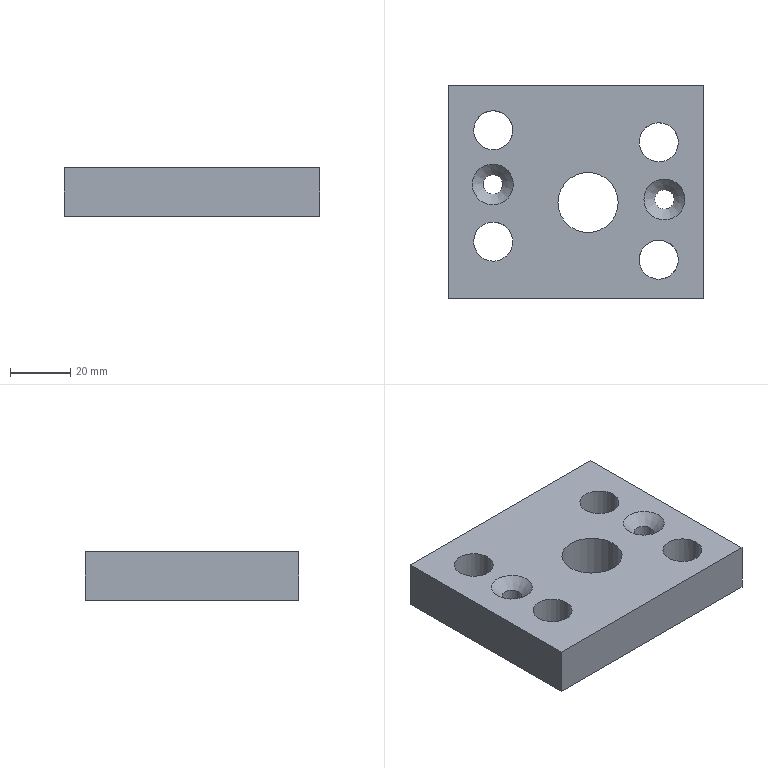Part | STEP file | gslz 2016.10.28-13_id1610_x_t | 1 solid | 15 faces | box 85 x 71 x 16 mm | volume 81626 mm3 | cylinder 7 | plane 6 | cone 2 | commonest cylinder face diameters 13 x4 6.5 x2 20 x1
STEP:
#1=CARTESIAN_POINT('',(0.,0.,0.));
#2=DIRECTION('',(0.,0.,1.));
#3=DIRECTION('',(1.,0.,0.));
#4=AXIS2_PLACEMENT_3D('',#1,#2,#3);
#5=CARTESIAN_POINT('',(-1398.441,280.34,-48.));
#6=VERTEX_POINT('',#5);
#7=CARTESIAN_POINT('',(-1399.872,274.,-48.));
#8=DIRECTION('',(0.,0.,1.));
#9=DIRECTION('',(0.2202,0.9754,0.));
#10=AXIS2_PLACEMENT_3D('',#7,#8,#9);
#11=CIRCLE('',#10,6.5);
#12=CARTESIAN_POINT('',(-1345.502,255.485,-48.));
#13=DIRECTION('',(0.,0.,1.));
#14=DIRECTION('',(1.,0.,0.));
#15=AXIS2_PLACEMENT_3D('',#12,#13,#14);
#16=PLANE('',#15);
#17=CARTESIAN_POINT('',(-54.371,18.515));
#18=DIRECTION('',(0.2202,0.9754));
#19=AXIS2_PLACEMENT_2D('',#17,#18);
#20=CIRCLE('',#19,6.5);
#21=(GEOMETRIC_REPRESENTATION_CONTEXT(2)PARAMETRIC_REPRESENTATION_CONTEXT()REPRESENTATION_CONTEXT('',''));
#22=DEFINITIONAL_REPRESENTATION('',(#20),#21);
#23=PCURVE('',#16,#22);
#24=CARTESIAN_POINT('',(-1399.872,274.,-95.));
#25=DIRECTION('',(0.,0.,1.));
#26=DIRECTION('',(-0.2202,-0.9754,0.));
#27=AXIS2_PLACEMENT_3D('',#24,#25,#26);
#28=CYLINDRICAL_SURFACE('',#27,6.5);
#29=CARTESIAN_POINT('',(3.142,47.));
#30=DIRECTION('',(1.,0.));
#31=VECTOR('',#30,1.);
#32=LINE('',#29,#31);
#33=(GEOMETRIC_REPRESENTATION_CONTEXT(2)PARAMETRIC_REPRESENTATION_CONTEXT()REPRESENTATION_CONTEXT('',''));
#34=DEFINITIONAL_REPRESENTATION('',(#32),#33);
#35=PCURVE('',#28,#34);
#36=SURFACE_CURVE('',#11,(#23,#35),.PCURVE_S1.);
#37=EDGE_CURVE('',#6,#6,#36,.T.);
#38=ORIENTED_EDGE('',*,*,#37,.T.);
#39=EDGE_LOOP('',(#38));
#40=FACE_BOUND('',#39,.T.);
#41=CARTESIAN_POINT('',(-1455.963,271.592,-48.));
#42=VERTEX_POINT('',#41);
#43=CARTESIAN_POINT('',(-1454.872,278.,-48.));
#44=DIRECTION('',(0.,0.,1.));
#45=DIRECTION('',(-0.1678,-0.9858,0.));
#46=AXIS2_PLACEMENT_3D('',#43,#44,#45);
#47=CIRCLE('',#46,6.5);
#48=CARTESIAN_POINT('',(-109.371,22.515));
#49=DIRECTION('',(-0.1678,-0.9858));
#50=AXIS2_PLACEMENT_2D('',#48,#49);
#51=CIRCLE('',#50,6.5);
#52=(GEOMETRIC_REPRESENTATION_CONTEXT(2)PARAMETRIC_REPRESENTATION_CONTEXT()REPRESENTATION_CONTEXT('',''));
#53=DEFINITIONAL_REPRESENTATION('',(#51),#52);
#54=PCURVE('',#16,#53);
#55=CARTESIAN_POINT('',(-1454.872,278.,-0.5408));
#56=DIRECTION('',(0.,0.,-1.));
#57=DIRECTION('',(-1.,0.,0.));
#58=AXIS2_PLACEMENT_3D('',#55,#56,#57);
#59=CYLINDRICAL_SURFACE('',#58,6.5);
#60=CARTESIAN_POINT('',(11.164,47.459));
#61=DIRECTION('',(-1.,0.));
#62=VECTOR('',#61,1.);
#63=LINE('',#60,#62);
#64=(GEOMETRIC_REPRESENTATION_CONTEXT(2)PARAMETRIC_REPRESENTATION_CONTEXT()REPRESENTATION_CONTEXT('',''));
#65=DEFINITIONAL_REPRESENTATION('',(#63),#64);
#66=PCURVE('',#59,#65);
#67=SURFACE_CURVE('',#47,(#54,#66),.PCURVE_S1.);
#68=EDGE_CURVE('',#42,#42,#67,.T.);
#69=ORIENTED_EDGE('',*,*,#68,.T.);
#70=EDGE_LOOP('',(#69));
#71=FACE_BOUND('',#70,.T.);
#72=CARTESIAN_POINT('',(-1394.75,255.,-48.));
#73=VERTEX_POINT('',#72);
#74=CARTESIAN_POINT('',(-1398.,255.,-48.));
#75=DIRECTION('',(0.,0.,-1.));
#76=DIRECTION('',(1.,0.,0.));
#77=AXIS2_PLACEMENT_3D('',#74,#75,#76);
#78=CIRCLE('',#77,3.25);
#79=CARTESIAN_POINT('',(-49.248,-0.4849));
#80=CARTESIAN_POINT('',(-49.248,-6.114));
#81=CARTESIAN_POINT('',(-54.123,-3.299));
#82=CARTESIAN_POINT('',(-58.998,-0.4849));
#83=CARTESIAN_POINT('',(-54.123,2.33));
#84=CARTESIAN_POINT('',(-49.248,5.144));
#85=CARTESIAN_POINT('',(-49.248,-0.4849));
#86=(BOUNDED_CURVE()B_SPLINE_CURVE(2,(#79,#80,#81,#82,#83,#84,#85),.UNSPECIFIED.,.T.,.F.)B_SPLINE_CURVE_WITH_KNOTS((1,2,2,2,2,1),(-2.094,0.,2.094,4.189,6.283,8.378),.UNSPECIFIED.)CURVE()GEOMETRIC_REPRESENTATION_ITEM()RATIONAL_B_SPLINE_CURVE((1.,0.5,1.,0.5,1.,0.5,1.))REPRESENTATION_ITEM(''));
#87=(GEOMETRIC_REPRESENTATION_CONTEXT(2)PARAMETRIC_REPRESENTATION_CONTEXT()REPRESENTATION_CONTEXT('',''));
#88=DEFINITIONAL_REPRESENTATION('',(#86),#87);
#89=PCURVE('',#16,#88);
#90=CARTESIAN_POINT('',(-1398.,255.,-32.));
#91=DIRECTION('',(0.,0.,-1.));
#92=DIRECTION('',(-1.,0.,0.));
#93=AXIS2_PLACEMENT_3D('',#90,#91,#92);
#94=CYLINDRICAL_SURFACE('',#93,3.25);
#95=CARTESIAN_POINT('',(3.142,16.));
#96=DIRECTION('',(1.,0.));
#97=VECTOR('',#96,1.);
#98=LINE('',#95,#97);
#99=(GEOMETRIC_REPRESENTATION_CONTEXT(2)PARAMETRIC_REPRESENTATION_CONTEXT()REPRESENTATION_CONTEXT('',''));
#100=DEFINITIONAL_REPRESENTATION('',(#98),#99);
#101=PCURVE('',#94,#100);
#102=SURFACE_CURVE('',#78,(#89,#101),.PCURVE_S1.);
#103=EDGE_CURVE('',#73,#73,#102,.T.);
#104=ORIENTED_EDGE('',*,*,#103,.F.);
#105=EDGE_LOOP('',(#104));
#106=FACE_BOUND('',#105,.T.);
#107=CARTESIAN_POINT('',(-1451.75,260.,-48.));
#108=VERTEX_POINT('',#107);
#109=CARTESIAN_POINT('',(-1455.,260.,-48.));
#110=DIRECTION('',(0.,0.,-1.));
#111=DIRECTION('',(1.,0.,0.));
#112=AXIS2_PLACEMENT_3D('',#109,#110,#111);
#113=CIRCLE('',#112,3.25);
#114=CARTESIAN_POINT('',(-106.248,4.515));
#115=CARTESIAN_POINT('',(-106.248,-1.114));
#116=CARTESIAN_POINT('',(-111.123,1.701));
#117=CARTESIAN_POINT('',(-115.998,4.515));
#118=CARTESIAN_POINT('',(-111.123,7.33));
#119=CARTESIAN_POINT('',(-106.248,10.144));
#120=CARTESIAN_POINT('',(-106.248,4.515));
#121=(BOUNDED_CURVE()B_SPLINE_CURVE(2,(#114,#115,#116,#117,#118,#119,#120),.UNSPECIFIED.,.T.,.F.)B_SPLINE_CURVE_WITH_KNOTS((1,2,2,2,2,1),(-2.094,0.,2.094,4.189,6.283,8.378),.UNSPECIFIED.)CURVE()GEOMETRIC_REPRESENTATION_ITEM()RATIONAL_B_SPLINE_CURVE((1.,0.5,1.,0.5,1.,0.5,1.))REPRESENTATION_ITEM(''));
#122=(GEOMETRIC_REPRESENTATION_CONTEXT(2)PARAMETRIC_REPRESENTATION_CONTEXT()REPRESENTATION_CONTEXT('',''));
#123=DEFINITIONAL_REPRESENTATION('',(#121),#122);
#124=PCURVE('',#16,#123);
#125=CARTESIAN_POINT('',(-1455.,260.,-32.));
#126=DIRECTION('',(0.,0.,-1.));
#127=DIRECTION('',(-1.,0.,0.));
#128=AXIS2_PLACEMENT_3D('',#125,#126,#127);
#129=CYLINDRICAL_SURFACE('',#128,3.25);
#130=CARTESIAN_POINT('',(3.142,16.));
#131=DIRECTION('',(1.,0.));
#132=VECTOR('',#131,1.);
#133=LINE('',#130,#132);
#134=(GEOMETRIC_REPRESENTATION_CONTEXT(2)PARAMETRIC_REPRESENTATION_CONTEXT()REPRESENTATION_CONTEXT('',''));
#135=DEFINITIONAL_REPRESENTATION('',(#133),#134);
#136=PCURVE('',#129,#135);
#137=SURFACE_CURVE('',#113,(#124,#136),.PCURVE_S1.);
#138=EDGE_CURVE('',#108,#108,#137,.T.);
#139=ORIENTED_EDGE('',*,*,#138,.F.);
#140=EDGE_LOOP('',(#139));
#141=FACE_BOUND('',#140,.T.);
#142=CARTESIAN_POINT('',(-1469.872,293.,-48.));
#143=VERTEX_POINT('',#142);
#144=CARTESIAN_POINT('',(-1469.872,222.,-48.));
#145=VERTEX_POINT('',#144);
#146=CARTESIAN_POINT('',(-1469.872,336.,-48.));
#147=DIRECTION('',(0.,-1.,0.));
#148=VECTOR('',#147,1.);
#149=LINE('',#146,#148);
#150=CARTESIAN_POINT('',(-124.371,80.515));
#151=DIRECTION('',(0.,-1.));
#152=VECTOR('',#151,1.);
#153=LINE('',#150,#152);
#154=(GEOMETRIC_REPRESENTATION_CONTEXT(2)PARAMETRIC_REPRESENTATION_CONTEXT()REPRESENTATION_CONTEXT('',''));
#155=DEFINITIONAL_REPRESENTATION('',(#153),#154);
#156=PCURVE('',#16,#155);
#157=CARTESIAN_POINT('',(-1469.872,336.,-40.));
#158=DIRECTION('',(-1.,0.,0.));
#159=DIRECTION('',(0.,0.,1.));
#160=AXIS2_PLACEMENT_3D('',#157,#158,#159);
#161=PLANE('',#160);
#162=CARTESIAN_POINT('',(-8.,0.));
#163=DIRECTION('',(0.,-1.));
#164=VECTOR('',#163,1.);
#165=LINE('',#162,#164);
#166=(GEOMETRIC_REPRESENTATION_CONTEXT(2)PARAMETRIC_REPRESENTATION_CONTEXT()REPRESENTATION_CONTEXT('',''));
#167=DEFINITIONAL_REPRESENTATION('',(#165),#166);
#168=PCURVE('',#161,#167);
#169=SURFACE_CURVE('',#149,(#156,#168),.PCURVE_S1.);
#170=EDGE_CURVE('',#143,#145,#169,.T.);
#171=ORIENTED_EDGE('',*,*,#170,.F.);
#172=CARTESIAN_POINT('',(-1384.872,293.,-48.));
#173=VERTEX_POINT('',#172);
#174=CARTESIAN_POINT('',(-1423.372,293.,-48.));
#175=DIRECTION('',(-1.,0.,0.));
#176=VECTOR('',#175,1.);
#177=LINE('',#174,#176);
#178=CARTESIAN_POINT('',(-77.871,37.515));
#179=DIRECTION('',(-1.,0.));
#180=VECTOR('',#179,1.);
#181=LINE('',#178,#180);
#182=(GEOMETRIC_REPRESENTATION_CONTEXT(2)PARAMETRIC_REPRESENTATION_CONTEXT()REPRESENTATION_CONTEXT('',''));
#183=DEFINITIONAL_REPRESENTATION('',(#181),#182);
#184=PCURVE('',#16,#183);
#185=CARTESIAN_POINT('',(-1423.372,293.,-40.));
#186=DIRECTION('',(0.,1.,0.));
#187=DIRECTION('',(0.,0.,1.));
#188=AXIS2_PLACEMENT_3D('',#185,#186,#187);
#189=PLANE('',#188);
#190=CARTESIAN_POINT('',(-8.,0.));
#191=DIRECTION('',(0.,-1.));
#192=VECTOR('',#191,1.);
#193=LINE('',#190,#192);
#194=(GEOMETRIC_REPRESENTATION_CONTEXT(2)PARAMETRIC_REPRESENTATION_CONTEXT()REPRESENTATION_CONTEXT('',''));
#195=DEFINITIONAL_REPRESENTATION('',(#193),#194);
#196=PCURVE('',#189,#195);
#197=SURFACE_CURVE('',#177,(#184,#196),.PCURVE_S1.);
#198=EDGE_CURVE('',#173,#143,#197,.T.);
#199=ORIENTED_EDGE('',*,*,#198,.F.);
#200=CARTESIAN_POINT('',(-1384.872,222.,-48.));
#201=VERTEX_POINT('',#200);
#202=CARTESIAN_POINT('',(-1384.872,336.,-48.));
#203=DIRECTION('',(0.,1.,0.));
#204=VECTOR('',#203,1.);
#205=LINE('',#202,#204);
#206=CARTESIAN_POINT('',(-39.371,80.515));
#207=DIRECTION('',(0.,1.));
#208=VECTOR('',#207,1.);
#209=LINE('',#206,#208);
#210=(GEOMETRIC_REPRESENTATION_CONTEXT(2)PARAMETRIC_REPRESENTATION_CONTEXT()REPRESENTATION_CONTEXT('',''));
#211=DEFINITIONAL_REPRESENTATION('',(#209),#210);
#212=PCURVE('',#16,#211);
#213=CARTESIAN_POINT('',(-1384.872,336.,-40.));
#214=DIRECTION('',(1.,0.,0.));
#215=DIRECTION('',(0.,0.,-1.));
#216=AXIS2_PLACEMENT_3D('',#213,#214,#215);
#217=PLANE('',#216);
#218=CARTESIAN_POINT('',(8.,0.));
#219=DIRECTION('',(0.,1.));
#220=VECTOR('',#219,1.);
#221=LINE('',#218,#220);
#222=(GEOMETRIC_REPRESENTATION_CONTEXT(2)PARAMETRIC_REPRESENTATION_CONTEXT()REPRESENTATION_CONTEXT('',''));
#223=DEFINITIONAL_REPRESENTATION('',(#221),#222);
#224=PCURVE('',#217,#223);
#225=SURFACE_CURVE('',#205,(#212,#224),.PCURVE_S1.);
#226=EDGE_CURVE('',#201,#173,#225,.T.);
#227=ORIENTED_EDGE('',*,*,#226,.F.);
#228=CARTESIAN_POINT('',(-1423.372,222.,-48.));
#229=DIRECTION('',(1.,0.,0.));
#230=VECTOR('',#229,1.);
#231=LINE('',#228,#230);
#232=CARTESIAN_POINT('',(-77.871,-33.485));
#233=DIRECTION('',(1.,0.));
#234=VECTOR('',#233,1.);
#235=LINE('',#232,#234);
#236=(GEOMETRIC_REPRESENTATION_CONTEXT(2)PARAMETRIC_REPRESENTATION_CONTEXT()REPRESENTATION_CONTEXT('',''));
#237=DEFINITIONAL_REPRESENTATION('',(#235),#236);
#238=PCURVE('',#16,#237);
#239=CARTESIAN_POINT('',(-1423.372,222.,-40.));
#240=DIRECTION('',(0.,-1.,0.));
#241=DIRECTION('',(0.,0.,-1.));
#242=AXIS2_PLACEMENT_3D('',#239,#240,#241);
#243=PLANE('',#242);
#244=CARTESIAN_POINT('',(8.,0.));
#245=DIRECTION('',(0.,1.));
#246=VECTOR('',#245,1.);
#247=LINE('',#244,#246);
#248=(GEOMETRIC_REPRESENTATION_CONTEXT(2)PARAMETRIC_REPRESENTATION_CONTEXT()REPRESENTATION_CONTEXT('',''));
#249=DEFINITIONAL_REPRESENTATION('',(#247),#248);
#250=PCURVE('',#243,#249);
#251=SURFACE_CURVE('',#231,(#238,#250),.PCURVE_S1.);
#252=EDGE_CURVE('',#145,#201,#251,.T.);
#253=ORIENTED_EDGE('',*,*,#252,.F.);
#254=EDGE_LOOP('',(#171,#199,#227,#253));
#255=FACE_BOUND('',#254,.T.);
#256=CARTESIAN_POINT('',(-1413.372,254.,-48.));
#257=VERTEX_POINT('',#256);
#258=CARTESIAN_POINT('',(-1423.372,254.,-48.));
#259=DIRECTION('',(0.,0.,-1.));
#260=DIRECTION('',(1.,0.,0.));
#261=AXIS2_PLACEMENT_3D('',#258,#259,#260);
#262=CIRCLE('',#261,10.);
#263=CARTESIAN_POINT('',(-67.871,-1.485));
#264=CARTESIAN_POINT('',(-67.871,-18.805));
#265=CARTESIAN_POINT('',(-82.871,-10.145));
#266=CARTESIAN_POINT('',(-97.871,-1.485));
#267=CARTESIAN_POINT('',(-82.871,7.175));
#268=CARTESIAN_POINT('',(-67.871,15.836));
#269=CARTESIAN_POINT('',(-67.871,-1.485));
#270=(BOUNDED_CURVE()B_SPLINE_CURVE(2,(#263,#264,#265,#266,#267,#268,#269),.UNSPECIFIED.,.T.,.F.)B_SPLINE_CURVE_WITH_KNOTS((1,2,2,2,2,1),(-2.094,0.,2.094,4.189,6.283,8.378),.UNSPECIFIED.)CURVE()GEOMETRIC_REPRESENTATION_ITEM()RATIONAL_B_SPLINE_CURVE((1.,0.5,1.,0.5,1.,0.5,1.))REPRESENTATION_ITEM(''));
#271=(GEOMETRIC_REPRESENTATION_CONTEXT(2)PARAMETRIC_REPRESENTATION_CONTEXT()REPRESENTATION_CONTEXT('',''));
#272=DEFINITIONAL_REPRESENTATION('',(#270),#271);
#273=PCURVE('',#16,#272);
#274=CARTESIAN_POINT('',(-1423.372,254.,-257.));
#275=DIRECTION('',(0.,0.,1.));
#276=DIRECTION('',(1.,0.,0.));
#277=AXIS2_PLACEMENT_3D('',#274,#275,#276);
#278=CYLINDRICAL_SURFACE('',#277,10.);
#279=CARTESIAN_POINT('',(6.283,209.));
#280=DIRECTION('',(-1.,0.));
#281=VECTOR('',#280,1.);
#282=LINE('',#279,#281);
#283=(GEOMETRIC_REPRESENTATION_CONTEXT(2)PARAMETRIC_REPRESENTATION_CONTEXT()REPRESENTATION_CONTEXT('',''));
#284=DEFINITIONAL_REPRESENTATION('',(#282),#283);
#285=PCURVE('',#278,#284);
#286=SURFACE_CURVE('',#262,(#273,#285),.PCURVE_S1.);
#287=EDGE_CURVE('',#257,#257,#286,.T.);
#288=ORIENTED_EDGE('',*,*,#287,.F.);
#289=EDGE_LOOP('',(#288));
#290=FACE_BOUND('',#289,.T.);
#291=CARTESIAN_POINT('',(-1453.441,247.34,-48.));
#292=VERTEX_POINT('',#291);
#293=CARTESIAN_POINT('',(-1454.872,241.,-48.));
#294=DIRECTION('',(0.,0.,1.));
#295=DIRECTION('',(0.2202,0.9754,0.));
#296=AXIS2_PLACEMENT_3D('',#293,#294,#295);
#297=CIRCLE('',#296,6.5);
#298=CARTESIAN_POINT('',(-109.371,-14.485));
#299=DIRECTION('',(0.2202,0.9754));
#300=AXIS2_PLACEMENT_2D('',#298,#299);
#301=CIRCLE('',#300,6.5);
#302=(GEOMETRIC_REPRESENTATION_CONTEXT(2)PARAMETRIC_REPRESENTATION_CONTEXT()REPRESENTATION_CONTEXT('',''));
#303=DEFINITIONAL_REPRESENTATION('',(#301),#302);
#304=PCURVE('',#16,#303);
#305=CARTESIAN_POINT('',(-1454.872,241.,-95.));
#306=DIRECTION('',(0.,0.,1.));
#307=DIRECTION('',(-0.2202,-0.9754,0.));
#308=AXIS2_PLACEMENT_3D('',#305,#306,#307);
#309=CYLINDRICAL_SURFACE('',#308,6.5);
#310=CARTESIAN_POINT('',(3.142,47.));
#311=DIRECTION('',(1.,0.));
#312=VECTOR('',#311,1.);
#313=LINE('',#310,#312);
#314=(GEOMETRIC_REPRESENTATION_CONTEXT(2)PARAMETRIC_REPRESENTATION_CONTEXT()REPRESENTATION_CONTEXT('',''));
#315=DEFINITIONAL_REPRESENTATION('',(#313),#314);
#316=PCURVE('',#309,#315);
#317=SURFACE_CURVE('',#297,(#304,#316),.PCURVE_S1.);
#318=EDGE_CURVE('',#292,#292,#317,.T.);
#319=ORIENTED_EDGE('',*,*,#318,.T.);
#320=EDGE_LOOP('',(#319));
#321=FACE_BOUND('',#320,.T.);
#322=CARTESIAN_POINT('',(-1400.963,228.592,-48.));
#323=VERTEX_POINT('',#322);
#324=CARTESIAN_POINT('',(-1399.872,235.,-48.));
#325=DIRECTION('',(0.,0.,1.));
#326=DIRECTION('',(-0.1678,-0.9858,0.));
#327=AXIS2_PLACEMENT_3D('',#324,#325,#326);
#328=CIRCLE('',#327,6.5);
#329=CARTESIAN_POINT('',(-54.371,-20.485));
#330=DIRECTION('',(-0.1678,-0.9858));
#331=AXIS2_PLACEMENT_2D('',#329,#330);
#332=CIRCLE('',#331,6.5);
#333=(GEOMETRIC_REPRESENTATION_CONTEXT(2)PARAMETRIC_REPRESENTATION_CONTEXT()REPRESENTATION_CONTEXT('',''));
#334=DEFINITIONAL_REPRESENTATION('',(#332),#333);
#335=PCURVE('',#16,#334);
#336=CARTESIAN_POINT('',(-1399.872,235.,-0.5408));
#337=DIRECTION('',(0.,0.,-1.));
#338=DIRECTION('',(-1.,0.,0.));
#339=AXIS2_PLACEMENT_3D('',#336,#337,#338);
#340=CYLINDRICAL_SURFACE('',#339,6.5);
#341=CARTESIAN_POINT('',(11.164,47.459));
#342=DIRECTION('',(-1.,0.));
#343=VECTOR('',#342,1.);
#344=LINE('',#341,#343);
#345=(GEOMETRIC_REPRESENTATION_CONTEXT(2)PARAMETRIC_REPRESENTATION_CONTEXT()REPRESENTATION_CONTEXT('',''));
#346=DEFINITIONAL_REPRESENTATION('',(#344),#345);
#347=PCURVE('',#340,#346);
#348=SURFACE_CURVE('',#328,(#335,#347),.PCURVE_S1.);
#349=EDGE_CURVE('',#323,#323,#348,.T.);
#350=ORIENTED_EDGE('',*,*,#349,.T.);
#351=EDGE_LOOP('',(#350));
#352=FACE_BOUND('',#351,.T.);
#353=ADVANCED_FACE('',(#40,#71,#106,#141,#255,#290,#321,#352),#16,.F.);
#354=CARTESIAN_POINT('',(-1393.372,235.,-32.));
#355=VERTEX_POINT('',#354);
#356=CARTESIAN_POINT('',(-1400.963,228.592,-32.));
#357=VERTEX_POINT('',#356);
#358=CARTESIAN_POINT('',(-1399.872,235.,-32.));
#359=DIRECTION('',(0.,0.,-1.));
#360=DIRECTION('',(1.,0.,0.));
#361=AXIS2_PLACEMENT_3D('',#358,#359,#360);
#362=CIRCLE('',#361,6.5);
#363=CARTESIAN_POINT('',(-1345.502,255.485,-32.));
#364=DIRECTION('',(0.,0.,1.));
#365=DIRECTION('',(1.,0.,0.));
#366=AXIS2_PLACEMENT_3D('',#363,#364,#365);
#367=PLANE('',#366);
#368=CARTESIAN_POINT('',(-47.871,-20.485));
#369=CARTESIAN_POINT('',(-47.871,-31.743));
#370=CARTESIAN_POINT('',(-57.621,-26.114));
#371=CARTESIAN_POINT('',(-67.371,-20.485));
#372=CARTESIAN_POINT('',(-57.621,-14.856));
#373=CARTESIAN_POINT('',(-47.871,-9.227));
#374=CARTESIAN_POINT('',(-47.871,-20.485));
#375=(BOUNDED_CURVE()B_SPLINE_CURVE(2,(#368,#369,#370,#371,#372,#373,#374),.UNSPECIFIED.,.T.,.F.)B_SPLINE_CURVE_WITH_KNOTS((1,2,2,2,2,1),(-2.094,0.,2.094,4.189,6.283,8.378),.UNSPECIFIED.)CURVE()GEOMETRIC_REPRESENTATION_ITEM()RATIONAL_B_SPLINE_CURVE((1.,0.5,1.,0.5,1.,0.5,1.))REPRESENTATION_ITEM(''));
#376=(GEOMETRIC_REPRESENTATION_CONTEXT(2)PARAMETRIC_REPRESENTATION_CONTEXT()REPRESENTATION_CONTEXT('',''));
#377=DEFINITIONAL_REPRESENTATION('',(#375),#376);
#378=PCURVE('',#367,#377);
#379=CARTESIAN_POINT('',(9.425,31.459));
#380=DIRECTION('',(1.,0.));
#381=VECTOR('',#380,1.);
#382=LINE('',#379,#381);
#383=(GEOMETRIC_REPRESENTATION_CONTEXT(2)PARAMETRIC_REPRESENTATION_CONTEXT()REPRESENTATION_CONTEXT('',''));
#384=DEFINITIONAL_REPRESENTATION('',(#382),#383);
#385=PCURVE('',#340,#384);
#386=SURFACE_CURVE('',#362,(#378,#385),.PCURVE_S1.);
#387=EDGE_CURVE('',#355,#357,#386,.T.);
#388=ORIENTED_EDGE('',*,*,#387,.T.);
#389=CARTESIAN_POINT('',(-1399.872,235.,-32.));
#390=DIRECTION('',(0.,0.,-1.));
#391=DIRECTION('',(1.,0.,0.));
#392=AXIS2_PLACEMENT_3D('',#389,#390,#391);
#393=CIRCLE('',#392,6.5);
#394=CARTESIAN_POINT('',(-47.871,-20.485));
#395=CARTESIAN_POINT('',(-47.871,-31.743));
#396=CARTESIAN_POINT('',(-57.621,-26.114));
#397=CARTESIAN_POINT('',(-67.371,-20.485));
#398=CARTESIAN_POINT('',(-57.621,-14.856));
#399=CARTESIAN_POINT('',(-47.871,-9.227));
#400=CARTESIAN_POINT('',(-47.871,-20.485));
#401=(BOUNDED_CURVE()B_SPLINE_CURVE(2,(#394,#395,#396,#397,#398,#399,#400),.UNSPECIFIED.,.T.,.F.)B_SPLINE_CURVE_WITH_KNOTS((1,2,2,2,2,1),(-2.094,0.,2.094,4.189,6.283,8.378),.UNSPECIFIED.)CURVE()GEOMETRIC_REPRESENTATION_ITEM()RATIONAL_B_SPLINE_CURVE((1.,0.5,1.,0.5,1.,0.5,1.))REPRESENTATION_ITEM(''));
#402=(GEOMETRIC_REPRESENTATION_CONTEXT(2)PARAMETRIC_REPRESENTATION_CONTEXT()REPRESENTATION_CONTEXT('',''));
#403=DEFINITIONAL_REPRESENTATION('',(#401),#402);
#404=PCURVE('',#367,#403);
#405=CARTESIAN_POINT('',(3.142,31.459));
#406=DIRECTION('',(1.,0.));
#407=VECTOR('',#406,1.);
#408=LINE('',#405,#407);
#409=(GEOMETRIC_REPRESENTATION_CONTEXT(2)PARAMETRIC_REPRESENTATION_CONTEXT()REPRESENTATION_CONTEXT('',''));
#410=DEFINITIONAL_REPRESENTATION('',(#408),#409);
#411=PCURVE('',#340,#410);
#412=SURFACE_CURVE('',#393,(#404,#411),.PCURVE_S1.);
#413=EDGE_CURVE('',#357,#355,#412,.T.);
#414=ORIENTED_EDGE('',*,*,#413,.T.);
#415=EDGE_LOOP('',(#388,#414));
#416=FACE_BOUND('',#415,.T.);
#417=CARTESIAN_POINT('',(-1398.441,280.34,-32.));
#418=VERTEX_POINT('',#417);
#419=CARTESIAN_POINT('',(-1399.872,274.,-32.));
#420=DIRECTION('',(0.,0.,-1.));
#421=DIRECTION('',(0.2202,0.9754,0.));
#422=AXIS2_PLACEMENT_3D('',#419,#420,#421);
#423=CIRCLE('',#422,6.5);
#424=CARTESIAN_POINT('',(-52.939,24.856));
#425=CARTESIAN_POINT('',(-41.957,22.376));
#426=CARTESIAN_POINT('',(-49.595,14.105));
#427=CARTESIAN_POINT('',(-57.234,5.834));
#428=CARTESIAN_POINT('',(-60.577,16.585));
#429=CARTESIAN_POINT('',(-63.921,27.335));
#430=CARTESIAN_POINT('',(-52.939,24.856));
#431=(BOUNDED_CURVE()B_SPLINE_CURVE(2,(#424,#425,#426,#427,#428,#429,#430),.UNSPECIFIED.,.T.,.F.)B_SPLINE_CURVE_WITH_KNOTS((1,2,2,2,2,1),(-2.094,0.,2.094,4.189,6.283,8.378),.UNSPECIFIED.)CURVE()GEOMETRIC_REPRESENTATION_ITEM()RATIONAL_B_SPLINE_CURVE((1.,0.5,1.,0.5,1.,0.5,1.))REPRESENTATION_ITEM(''));
#432=(GEOMETRIC_REPRESENTATION_CONTEXT(2)PARAMETRIC_REPRESENTATION_CONTEXT()REPRESENTATION_CONTEXT('',''));
#433=DEFINITIONAL_REPRESENTATION('',(#431),#432);
#434=PCURVE('',#367,#433);
#435=CARTESIAN_POINT('',(9.425,63.));
#436=DIRECTION('',(-1.,0.));
#437=VECTOR('',#436,1.);
#438=LINE('',#435,#437);
#439=(GEOMETRIC_REPRESENTATION_CONTEXT(2)PARAMETRIC_REPRESENTATION_CONTEXT()REPRESENTATION_CONTEXT('',''));
#440=DEFINITIONAL_REPRESENTATION('',(#438),#439);
#441=PCURVE('',#28,#440);
#442=SURFACE_CURVE('',#423,(#434,#441),.PCURVE_S1.);
#443=EDGE_CURVE('',#418,#418,#442,.T.);
#444=ORIENTED_EDGE('',*,*,#443,.T.);
#445=EDGE_LOOP('',(#444));
#446=FACE_BOUND('',#445,.T.);
#447=CARTESIAN_POINT('',(-1448.372,278.,-32.));
#448=VERTEX_POINT('',#447);
#449=CARTESIAN_POINT('',(-1455.963,271.592,-32.));
#450=VERTEX_POINT('',#449);
#451=CARTESIAN_POINT('',(-1454.872,278.,-32.));
#452=DIRECTION('',(0.,0.,-1.));
#453=DIRECTION('',(1.,0.,0.));
#454=AXIS2_PLACEMENT_3D('',#451,#452,#453);
#455=CIRCLE('',#454,6.5);
#456=CARTESIAN_POINT('',(-102.871,22.515));
#457=CARTESIAN_POINT('',(-102.871,11.257));
#458=CARTESIAN_POINT('',(-112.621,16.886));
#459=CARTESIAN_POINT('',(-122.371,22.515));
#460=CARTESIAN_POINT('',(-112.621,28.144));
#461=CARTESIAN_POINT('',(-102.871,33.773));
#462=CARTESIAN_POINT('',(-102.871,22.515));
#463=(BOUNDED_CURVE()B_SPLINE_CURVE(2,(#456,#457,#458,#459,#460,#461,#462),.UNSPECIFIED.,.T.,.F.)B_SPLINE_CURVE_WITH_KNOTS((1,2,2,2,2,1),(-2.094,0.,2.094,4.189,6.283,8.378),.UNSPECIFIED.)CURVE()GEOMETRIC_REPRESENTATION_ITEM()RATIONAL_B_SPLINE_CURVE((1.,0.5,1.,0.5,1.,0.5,1.))REPRESENTATION_ITEM(''));
#464=(GEOMETRIC_REPRESENTATION_CONTEXT(2)PARAMETRIC_REPRESENTATION_CONTEXT()REPRESENTATION_CONTEXT('',''));
#465=DEFINITIONAL_REPRESENTATION('',(#463),#464);
#466=PCURVE('',#367,#465);
#467=CARTESIAN_POINT('',(9.425,31.459));
#468=DIRECTION('',(1.,0.));
#469=VECTOR('',#468,1.);
#470=LINE('',#467,#469);
#471=(GEOMETRIC_REPRESENTATION_CONTEXT(2)PARAMETRIC_REPRESENTATION_CONTEXT()REPRESENTATION_CONTEXT('',''));
#472=DEFINITIONAL_REPRESENTATION('',(#470),#471);
#473=PCURVE('',#59,#472);
#474=SURFACE_CURVE('',#455,(#466,#473),.PCURVE_S1.);
#475=EDGE_CURVE('',#448,#450,#474,.T.);
#476=ORIENTED_EDGE('',*,*,#475,.T.);
#477=CARTESIAN_POINT('',(-1454.872,278.,-32.));
#478=DIRECTION('',(0.,0.,-1.));
#479=DIRECTION('',(1.,0.,0.));
#480=AXIS2_PLACEMENT_3D('',#477,#478,#479);
#481=CIRCLE('',#480,6.5);
#482=CARTESIAN_POINT('',(-102.871,22.515));
#483=CARTESIAN_POINT('',(-102.871,11.257));
#484=CARTESIAN_POINT('',(-112.621,16.886));
#485=CARTESIAN_POINT('',(-122.371,22.515));
#486=CARTESIAN_POINT('',(-112.621,28.144));
#487=CARTESIAN_POINT('',(-102.871,33.773));
#488=CARTESIAN_POINT('',(-102.871,22.515));
#489=(BOUNDED_CURVE()B_SPLINE_CURVE(2,(#482,#483,#484,#485,#486,#487,#488),.UNSPECIFIED.,.T.,.F.)B_SPLINE_CURVE_WITH_KNOTS((1,2,2,2,2,1),(-2.094,0.,2.094,4.189,6.283,8.378),.UNSPECIFIED.)CURVE()GEOMETRIC_REPRESENTATION_ITEM()RATIONAL_B_SPLINE_CURVE((1.,0.5,1.,0.5,1.,0.5,1.))REPRESENTATION_ITEM(''));
#490=(GEOMETRIC_REPRESENTATION_CONTEXT(2)PARAMETRIC_REPRESENTATION_CONTEXT()REPRESENTATION_CONTEXT('',''));
#491=DEFINITIONAL_REPRESENTATION('',(#489),#490);
#492=PCURVE('',#367,#491);
#493=CARTESIAN_POINT('',(3.142,31.459));
#494=DIRECTION('',(1.,0.));
#495=VECTOR('',#494,1.);
#496=LINE('',#493,#495);
#497=(GEOMETRIC_REPRESENTATION_CONTEXT(2)PARAMETRIC_REPRESENTATION_CONTEXT()REPRESENTATION_CONTEXT('',''));
#498=DEFINITIONAL_REPRESENTATION('',(#496),#497);
#499=PCURVE('',#59,#498);
#500=SURFACE_CURVE('',#481,(#492,#499),.PCURVE_S1.);
#501=EDGE_CURVE('',#450,#448,#500,.T.);
#502=ORIENTED_EDGE('',*,*,#501,.T.);
#503=EDGE_LOOP('',(#476,#502));
#504=FACE_BOUND('',#503,.T.);
#505=CARTESIAN_POINT('',(-1461.8,260.,-32.));
#506=VERTEX_POINT('',#505);
#507=CARTESIAN_POINT('',(-1455.,260.,-32.));
#508=DIRECTION('',(0.,0.,1.));
#509=DIRECTION('',(-1.,0.,0.));
#510=AXIS2_PLACEMENT_3D('',#507,#508,#509);
#511=CIRCLE('',#510,6.8);
#512=CARTESIAN_POINT('',(-109.498,4.515));
#513=DIRECTION('',(-1.,0.));
#514=AXIS2_PLACEMENT_2D('',#512,#513);
#515=CIRCLE('',#514,6.8);
#516=(GEOMETRIC_REPRESENTATION_CONTEXT(2)PARAMETRIC_REPRESENTATION_CONTEXT()REPRESENTATION_CONTEXT('',''));
#517=DEFINITIONAL_REPRESENTATION('',(#515),#516);
#518=PCURVE('',#367,#517);
#519=CARTESIAN_POINT('',(-1455.,260.,-35.8));
#520=DIRECTION('',(0.,0.,1.));
#521=DIRECTION('',(-1.,0.,0.));
#522=AXIS2_PLACEMENT_3D('',#519,#520,#521);
#523=CONICAL_SURFACE('',#522,3.,0.7854);
#524=CARTESIAN_POINT('',(0.,3.8));
#525=DIRECTION('',(1.,0.));
#526=VECTOR('',#525,1.);
#527=LINE('',#524,#526);
#528=(GEOMETRIC_REPRESENTATION_CONTEXT(2)PARAMETRIC_REPRESENTATION_CONTEXT()REPRESENTATION_CONTEXT('',''));
#529=DEFINITIONAL_REPRESENTATION('',(#527),#528);
#530=PCURVE('',#523,#529);
#531=SURFACE_CURVE('',#511,(#518,#530),.PCURVE_S1.);
#532=EDGE_CURVE('',#506,#506,#531,.T.);
#533=ORIENTED_EDGE('',*,*,#532,.F.);
#534=EDGE_LOOP('',(#533));
#535=FACE_BOUND('',#534,.T.);
#536=CARTESIAN_POINT('',(-1384.872,293.,-32.));
#537=VERTEX_POINT('',#536);
#538=CARTESIAN_POINT('',(-1469.872,293.,-32.));
#539=VERTEX_POINT('',#538);
#540=CARTESIAN_POINT('',(-1423.372,293.,-32.));
#541=DIRECTION('',(-1.,0.,0.));
#542=VECTOR('',#541,1.);
#543=LINE('',#540,#542);
#544=CARTESIAN_POINT('',(-77.871,37.515));
#545=DIRECTION('',(-1.,0.));
#546=VECTOR('',#545,1.);
#547=LINE('',#544,#546);
#548=(GEOMETRIC_REPRESENTATION_CONTEXT(2)PARAMETRIC_REPRESENTATION_CONTEXT()REPRESENTATION_CONTEXT('',''));
#549=DEFINITIONAL_REPRESENTATION('',(#547),#548);
#550=PCURVE('',#367,#549);
#551=CARTESIAN_POINT('',(8.,0.));
#552=DIRECTION('',(0.,-1.));
#553=VECTOR('',#552,1.);
#554=LINE('',#551,#553);
#555=(GEOMETRIC_REPRESENTATION_CONTEXT(2)PARAMETRIC_REPRESENTATION_CONTEXT()REPRESENTATION_CONTEXT('',''));
#556=DEFINITIONAL_REPRESENTATION('',(#554),#555);
#557=PCURVE('',#189,#556);
#558=SURFACE_CURVE('',#543,(#550,#557),.PCURVE_S1.);
#559=EDGE_CURVE('',#537,#539,#558,.T.);
#560=ORIENTED_EDGE('',*,*,#559,.T.);
#561=CARTESIAN_POINT('',(-1469.872,222.,-32.));
#562=VERTEX_POINT('',#561);
#563=CARTESIAN_POINT('',(-1469.872,336.,-32.));
#564=DIRECTION('',(0.,-1.,0.));
#565=VECTOR('',#564,1.);
#566=LINE('',#563,#565);
#567=CARTESIAN_POINT('',(-124.371,80.515));
#568=DIRECTION('',(0.,-1.));
#569=VECTOR('',#568,1.);
#570=LINE('',#567,#569);
#571=(GEOMETRIC_REPRESENTATION_CONTEXT(2)PARAMETRIC_REPRESENTATION_CONTEXT()REPRESENTATION_CONTEXT('',''));
#572=DEFINITIONAL_REPRESENTATION('',(#570),#571);
#573=PCURVE('',#367,#572);
#574=CARTESIAN_POINT('',(8.,0.));
#575=DIRECTION('',(0.,-1.));
#576=VECTOR('',#575,1.);
#577=LINE('',#574,#576);
#578=(GEOMETRIC_REPRESENTATION_CONTEXT(2)PARAMETRIC_REPRESENTATION_CONTEXT()REPRESENTATION_CONTEXT('',''));
#579=DEFINITIONAL_REPRESENTATION('',(#577),#578);
#580=PCURVE('',#161,#579);
#581=SURFACE_CURVE('',#566,(#573,#580),.PCURVE_S1.);
#582=EDGE_CURVE('',#539,#562,#581,.T.);
#583=ORIENTED_EDGE('',*,*,#582,.T.);
#584=CARTESIAN_POINT('',(-1384.872,222.,-32.));
#585=VERTEX_POINT('',#584);
#586=CARTESIAN_POINT('',(-1423.372,222.,-32.));
#587=DIRECTION('',(1.,0.,0.));
#588=VECTOR('',#587,1.);
#589=LINE('',#586,#588);
#590=CARTESIAN_POINT('',(-77.871,-33.485));
#591=DIRECTION('',(1.,0.));
#592=VECTOR('',#591,1.);
#593=LINE('',#590,#592);
#594=(GEOMETRIC_REPRESENTATION_CONTEXT(2)PARAMETRIC_REPRESENTATION_CONTEXT()REPRESENTATION_CONTEXT('',''));
#595=DEFINITIONAL_REPRESENTATION('',(#593),#594);
#596=PCURVE('',#367,#595);
#597=CARTESIAN_POINT('',(-8.,0.));
#598=DIRECTION('',(0.,1.));
#599=VECTOR('',#598,1.);
#600=LINE('',#597,#599);
#601=(GEOMETRIC_REPRESENTATION_CONTEXT(2)PARAMETRIC_REPRESENTATION_CONTEXT()REPRESENTATION_CONTEXT('',''));
#602=DEFINITIONAL_REPRESENTATION('',(#600),#601);
#603=PCURVE('',#243,#602);
#604=SURFACE_CURVE('',#589,(#596,#603),.PCURVE_S1.);
#605=EDGE_CURVE('',#562,#585,#604,.T.);
#606=ORIENTED_EDGE('',*,*,#605,.T.);
#607=CARTESIAN_POINT('',(-1384.872,336.,-32.));
#608=DIRECTION('',(0.,1.,0.));
#609=VECTOR('',#608,1.);
#610=LINE('',#607,#609);
#611=CARTESIAN_POINT('',(-39.371,80.515));
#612=DIRECTION('',(0.,1.));
#613=VECTOR('',#612,1.);
#614=LINE('',#611,#613);
#615=(GEOMETRIC_REPRESENTATION_CONTEXT(2)PARAMETRIC_REPRESENTATION_CONTEXT()REPRESENTATION_CONTEXT('',''));
#616=DEFINITIONAL_REPRESENTATION('',(#614),#615);
#617=PCURVE('',#367,#616);
#618=CARTESIAN_POINT('',(-8.,0.));
#619=DIRECTION('',(0.,1.));
#620=VECTOR('',#619,1.);
#621=LINE('',#618,#620);
#622=(GEOMETRIC_REPRESENTATION_CONTEXT(2)PARAMETRIC_REPRESENTATION_CONTEXT()REPRESENTATION_CONTEXT('',''));
#623=DEFINITIONAL_REPRESENTATION('',(#621),#622);
#624=PCURVE('',#217,#623);
#625=SURFACE_CURVE('',#610,(#617,#624),.PCURVE_S1.);
#626=EDGE_CURVE('',#585,#537,#625,.T.);
#627=ORIENTED_EDGE('',*,*,#626,.T.);
#628=EDGE_LOOP('',(#560,#583,#606,#627));
#629=FACE_BOUND('',#628,.T.);
#630=CARTESIAN_POINT('',(-1413.372,254.,-32.));
#631=VERTEX_POINT('',#630);
#632=CARTESIAN_POINT('',(-1423.372,254.,-32.));
#633=DIRECTION('',(0.,0.,-1.));
#634=DIRECTION('',(1.,0.,0.));
#635=AXIS2_PLACEMENT_3D('',#632,#633,#634);
#636=CIRCLE('',#635,10.);
#637=CARTESIAN_POINT('',(-67.871,-1.485));
#638=CARTESIAN_POINT('',(-67.871,-18.805));
#639=CARTESIAN_POINT('',(-82.871,-10.145));
#640=CARTESIAN_POINT('',(-97.871,-1.485));
#641=CARTESIAN_POINT('',(-82.871,7.175));
#642=CARTESIAN_POINT('',(-67.871,15.836));
#643=CARTESIAN_POINT('',(-67.871,-1.485));
#644=(BOUNDED_CURVE()B_SPLINE_CURVE(2,(#637,#638,#639,#640,#641,#642,#643),.UNSPECIFIED.,.T.,.F.)B_SPLINE_CURVE_WITH_KNOTS((1,2,2,2,2,1),(-2.094,0.,2.094,4.189,6.283,8.378),.UNSPECIFIED.)CURVE()GEOMETRIC_REPRESENTATION_ITEM()RATIONAL_B_SPLINE_CURVE((1.,0.5,1.,0.5,1.,0.5,1.))REPRESENTATION_ITEM(''));
#645=(GEOMETRIC_REPRESENTATION_CONTEXT(2)PARAMETRIC_REPRESENTATION_CONTEXT()REPRESENTATION_CONTEXT('',''));
#646=DEFINITIONAL_REPRESENTATION('',(#644),#645);
#647=PCURVE('',#367,#646);
#648=CARTESIAN_POINT('',(6.283,225.));
#649=DIRECTION('',(-1.,0.));
#650=VECTOR('',#649,1.);
#651=LINE('',#648,#650);
#652=(GEOMETRIC_REPRESENTATION_CONTEXT(2)PARAMETRIC_REPRESENTATION_CONTEXT()REPRESENTATION_CONTEXT('',''));
#653=DEFINITIONAL_REPRESENTATION('',(#651),#652);
#654=PCURVE('',#278,#653);
#655=SURFACE_CURVE('',#636,(#647,#654),.PCURVE_S1.);
#656=EDGE_CURVE('',#631,#631,#655,.T.);
#657=ORIENTED_EDGE('',*,*,#656,.T.);
#658=EDGE_LOOP('',(#657));
#659=FACE_BOUND('',#658,.T.);
#660=CARTESIAN_POINT('',(-1404.8,255.,-32.));
#661=VERTEX_POINT('',#660);
#662=CARTESIAN_POINT('',(-1398.,255.,-32.));
#663=DIRECTION('',(0.,0.,1.));
#664=DIRECTION('',(-1.,0.,0.));
#665=AXIS2_PLACEMENT_3D('',#662,#663,#664);
#666=CIRCLE('',#665,6.8);
#667=CARTESIAN_POINT('',(-52.498,-0.4849));
#668=DIRECTION('',(-1.,0.));
#669=AXIS2_PLACEMENT_2D('',#667,#668);
#670=CIRCLE('',#669,6.8);
#671=(GEOMETRIC_REPRESENTATION_CONTEXT(2)PARAMETRIC_REPRESENTATION_CONTEXT()REPRESENTATION_CONTEXT('',''));
#672=DEFINITIONAL_REPRESENTATION('',(#670),#671);
#673=PCURVE('',#367,#672);
#674=CARTESIAN_POINT('',(-1398.,255.,-35.8));
#675=DIRECTION('',(0.,0.,1.));
#676=DIRECTION('',(-1.,0.,0.));
#677=AXIS2_PLACEMENT_3D('',#674,#675,#676);
#678=CONICAL_SURFACE('',#677,3.,0.7854);
#679=CARTESIAN_POINT('',(0.,3.8));
#680=DIRECTION('',(1.,0.));
#681=VECTOR('',#680,1.);
#682=LINE('',#679,#681);
#683=(GEOMETRIC_REPRESENTATION_CONTEXT(2)PARAMETRIC_REPRESENTATION_CONTEXT()REPRESENTATION_CONTEXT('',''));
#684=DEFINITIONAL_REPRESENTATION('',(#682),#683);
#685=PCURVE('',#678,#684);
#686=SURFACE_CURVE('',#666,(#673,#685),.PCURVE_S1.);
#687=EDGE_CURVE('',#661,#661,#686,.T.);
#688=ORIENTED_EDGE('',*,*,#687,.F.);
#689=EDGE_LOOP('',(#688));
#690=FACE_BOUND('',#689,.T.);
#691=CARTESIAN_POINT('',(-1453.441,247.34,-32.));
#692=VERTEX_POINT('',#691);
#693=CARTESIAN_POINT('',(-1454.872,241.,-32.));
#694=DIRECTION('',(0.,0.,-1.));
#695=DIRECTION('',(0.2202,0.9754,0.));
#696=AXIS2_PLACEMENT_3D('',#693,#694,#695);
#697=CIRCLE('',#696,6.5);
#698=CARTESIAN_POINT('',(-107.939,-8.144));
#699=CARTESIAN_POINT('',(-96.957,-10.624));
#700=CARTESIAN_POINT('',(-104.595,-18.895));
#701=CARTESIAN_POINT('',(-112.234,-27.166));
#702=CARTESIAN_POINT('',(-115.577,-16.415));
#703=CARTESIAN_POINT('',(-118.921,-5.665));
#704=CARTESIAN_POINT('',(-107.939,-8.144));
#705=(BOUNDED_CURVE()B_SPLINE_CURVE(2,(#698,#699,#700,#701,#702,#703,#704),.UNSPECIFIED.,.T.,.F.)B_SPLINE_CURVE_WITH_KNOTS((1,2,2,2,2,1),(-2.094,0.,2.094,4.189,6.283,8.378),.UNSPECIFIED.)CURVE()GEOMETRIC_REPRESENTATION_ITEM()RATIONAL_B_SPLINE_CURVE((1.,0.5,1.,0.5,1.,0.5,1.))REPRESENTATION_ITEM(''));
#706=(GEOMETRIC_REPRESENTATION_CONTEXT(2)PARAMETRIC_REPRESENTATION_CONTEXT()REPRESENTATION_CONTEXT('',''));
#707=DEFINITIONAL_REPRESENTATION('',(#705),#706);
#708=PCURVE('',#367,#707);
#709=CARTESIAN_POINT('',(9.425,63.));
#710=DIRECTION('',(-1.,0.));
#711=VECTOR('',#710,1.);
#712=LINE('',#709,#711);
#713=(GEOMETRIC_REPRESENTATION_CONTEXT(2)PARAMETRIC_REPRESENTATION_CONTEXT()REPRESENTATION_CONTEXT('',''));
#714=DEFINITIONAL_REPRESENTATION('',(#712),#713);
#715=PCURVE('',#309,#714);
#716=SURFACE_CURVE('',#697,(#708,#715),.PCURVE_S1.);
#717=EDGE_CURVE('',#692,#692,#716,.T.);
#718=ORIENTED_EDGE('',*,*,#717,.T.);
#719=EDGE_LOOP('',(#718));
#720=FACE_BOUND('',#719,.T.);
#721=ADVANCED_FACE('',(#416,#446,#504,#535,#629,#659,#690,#720),#367,.T.);
#722=ORIENTED_EDGE('',*,*,#198,.T.);
#723=CARTESIAN_POINT('',(-1469.872,293.,-40.));
#724=DIRECTION('',(0.,0.,1.));
#725=VECTOR('',#724,1.);
#726=LINE('',#723,#725);
#727=CARTESIAN_POINT('',(0.,-46.5));
#728=DIRECTION('',(1.,0.));
#729=VECTOR('',#728,1.);
#730=LINE('',#727,#729);
#731=(GEOMETRIC_REPRESENTATION_CONTEXT(2)PARAMETRIC_REPRESENTATION_CONTEXT()REPRESENTATION_CONTEXT('',''));
#732=DEFINITIONAL_REPRESENTATION('',(#730),#731);
#733=PCURVE('',#189,#732);
#734=CARTESIAN_POINT('',(0.,-43.));
#735=DIRECTION('',(1.,0.));
#736=VECTOR('',#735,1.);
#737=LINE('',#734,#736);
#738=(GEOMETRIC_REPRESENTATION_CONTEXT(2)PARAMETRIC_REPRESENTATION_CONTEXT()REPRESENTATION_CONTEXT('',''));
#739=DEFINITIONAL_REPRESENTATION('',(#737),#738);
#740=PCURVE('',#161,#739);
#741=SURFACE_CURVE('',#726,(#733,#740),.PCURVE_S1.);
#742=EDGE_CURVE('',#143,#539,#741,.T.);
#743=ORIENTED_EDGE('',*,*,#742,.T.);
#744=ORIENTED_EDGE('',*,*,#559,.F.);
#745=CARTESIAN_POINT('',(-1384.872,293.,-40.));
#746=DIRECTION('',(0.,0.,-1.));
#747=VECTOR('',#746,1.);
#748=LINE('',#745,#747);
#749=CARTESIAN_POINT('',(0.,38.5));
#750=DIRECTION('',(-1.,0.));
#751=VECTOR('',#750,1.);
#752=LINE('',#749,#751);
#753=(GEOMETRIC_REPRESENTATION_CONTEXT(2)PARAMETRIC_REPRESENTATION_CONTEXT()REPRESENTATION_CONTEXT('',''));
#754=DEFINITIONAL_REPRESENTATION('',(#752),#753);
#755=PCURVE('',#189,#754);
#756=CARTESIAN_POINT('',(0.,-43.));
#757=DIRECTION('',(1.,0.));
#758=VECTOR('',#757,1.);
#759=LINE('',#756,#758);
#760=(GEOMETRIC_REPRESENTATION_CONTEXT(2)PARAMETRIC_REPRESENTATION_CONTEXT()REPRESENTATION_CONTEXT('',''));
#761=DEFINITIONAL_REPRESENTATION('',(#759),#760);
#762=PCURVE('',#217,#761);
#763=SURFACE_CURVE('',#748,(#755,#762),.PCURVE_S1.);
#764=EDGE_CURVE('',#537,#173,#763,.T.);
#765=ORIENTED_EDGE('',*,*,#764,.T.);
#766=EDGE_LOOP('',(#722,#743,#744,#765));
#767=FACE_BOUND('',#766,.T.);
#768=ADVANCED_FACE('',(#767),#189,.T.);
#769=ORIENTED_EDGE('',*,*,#626,.F.);
#770=CARTESIAN_POINT('',(-1384.872,222.,-40.));
#771=DIRECTION('',(0.,0.,1.));
#772=VECTOR('',#771,1.);
#773=LINE('',#770,#772);
#774=CARTESIAN_POINT('',(0.,-114.));
#775=DIRECTION('',(-1.,0.));
#776=VECTOR('',#775,1.);
#777=LINE('',#774,#776);
#778=(GEOMETRIC_REPRESENTATION_CONTEXT(2)PARAMETRIC_REPRESENTATION_CONTEXT()REPRESENTATION_CONTEXT('',''));
#779=DEFINITIONAL_REPRESENTATION('',(#777),#778);
#780=PCURVE('',#217,#779);
#781=CARTESIAN_POINT('',(0.,38.5));
#782=DIRECTION('',(-1.,0.));
#783=VECTOR('',#782,1.);
#784=LINE('',#781,#783);
#785=(GEOMETRIC_REPRESENTATION_CONTEXT(2)PARAMETRIC_REPRESENTATION_CONTEXT()REPRESENTATION_CONTEXT('',''));
#786=DEFINITIONAL_REPRESENTATION('',(#784),#785);
#787=PCURVE('',#243,#786);
#788=SURFACE_CURVE('',#773,(#780,#787),.PCURVE_S1.);
#789=EDGE_CURVE('',#201,#585,#788,.T.);
#790=ORIENTED_EDGE('',*,*,#789,.F.);
#791=ORIENTED_EDGE('',*,*,#226,.T.);
#792=ORIENTED_EDGE('',*,*,#764,.F.);
#793=EDGE_LOOP('',(#769,#790,#791,#792));
#794=FACE_BOUND('',#793,.T.);
#795=ADVANCED_FACE('',(#794),#217,.T.);
#796=ORIENTED_EDGE('',*,*,#582,.F.);
#797=ORIENTED_EDGE('',*,*,#742,.F.);
#798=ORIENTED_EDGE('',*,*,#170,.T.);
#799=CARTESIAN_POINT('',(-1469.872,222.,-40.));
#800=DIRECTION('',(0.,0.,1.));
#801=VECTOR('',#800,1.);
#802=LINE('',#799,#801);
#803=CARTESIAN_POINT('',(0.,-114.));
#804=DIRECTION('',(1.,0.));
#805=VECTOR('',#804,1.);
#806=LINE('',#803,#805);
#807=(GEOMETRIC_REPRESENTATION_CONTEXT(2)PARAMETRIC_REPRESENTATION_CONTEXT()REPRESENTATION_CONTEXT('',''));
#808=DEFINITIONAL_REPRESENTATION('',(#806),#807);
#809=PCURVE('',#161,#808);
#810=CARTESIAN_POINT('',(0.,-46.5));
#811=DIRECTION('',(-1.,0.));
#812=VECTOR('',#811,1.);
#813=LINE('',#810,#812);
#814=(GEOMETRIC_REPRESENTATION_CONTEXT(2)PARAMETRIC_REPRESENTATION_CONTEXT()REPRESENTATION_CONTEXT('',''));
#815=DEFINITIONAL_REPRESENTATION('',(#813),#814);
#816=PCURVE('',#243,#815);
#817=SURFACE_CURVE('',#802,(#809,#816),.PCURVE_S1.);
#818=EDGE_CURVE('',#145,#562,#817,.T.);
#819=ORIENTED_EDGE('',*,*,#818,.T.);
#820=EDGE_LOOP('',(#796,#797,#798,#819));
#821=FACE_BOUND('',#820,.T.);
#822=ADVANCED_FACE('',(#821),#161,.T.);
#823=ORIENTED_EDGE('',*,*,#287,.F.);
#824=CARTESIAN_POINT('',(-1413.372,254.,-48.));
#825=CARTESIAN_POINT('',(-1413.372,254.,-32.));
#826=B_SPLINE_CURVE_WITH_KNOTS('',1,(#824,#825),.UNSPECIFIED.,.F.,.F.,(2,2),(209.,225.),.PIECEWISE_BEZIER_KNOTS.);
#827=CARTESIAN_POINT('',(6.283,0.));
#828=DIRECTION('',(0.,1.));
#829=VECTOR('',#828,1.);
#830=LINE('',#827,#829);
#831=(GEOMETRIC_REPRESENTATION_CONTEXT(2)PARAMETRIC_REPRESENTATION_CONTEXT()REPRESENTATION_CONTEXT('',''));
#832=DEFINITIONAL_REPRESENTATION('',(#830),#831);
#833=PCURVE('',#278,#832);
#834=CARTESIAN_POINT('',(0.,0.));
#835=DIRECTION('',(0.,1.));
#836=VECTOR('',#835,1.);
#837=LINE('',#834,#836);
#838=(GEOMETRIC_REPRESENTATION_CONTEXT(2)PARAMETRIC_REPRESENTATION_CONTEXT()REPRESENTATION_CONTEXT('',''));
#839=DEFINITIONAL_REPRESENTATION('',(#837),#838);
#840=PCURVE('',#278,#839);
#841=SEAM_CURVE('',#826,(#833,#840),.PCURVE_S1.);
#842=EDGE_CURVE('',#257,#631,#841,.T.);
#843=ORIENTED_EDGE('',*,*,#842,.T.);
#844=ORIENTED_EDGE('',*,*,#656,.T.);
#845=ORIENTED_EDGE('',*,*,#842,.F.);
#846=EDGE_LOOP('',(#823,#843,#844,#845));
#847=FACE_BOUND('',#846,.F.);
#848=ADVANCED_FACE('',(#847),#278,.F.);
#849=ORIENTED_EDGE('',*,*,#252,.T.);
#850=ORIENTED_EDGE('',*,*,#789,.T.);
#851=ORIENTED_EDGE('',*,*,#605,.F.);
#852=ORIENTED_EDGE('',*,*,#818,.F.);
#853=EDGE_LOOP('',(#849,#850,#851,#852));
#854=FACE_BOUND('',#853,.T.);
#855=ADVANCED_FACE('',(#854),#243,.T.);
#856=ORIENTED_EDGE('',*,*,#532,.F.);
#857=CARTESIAN_POINT('',(-1458.25,260.,-35.55));
#858=VERTEX_POINT('',#857);
#859=CARTESIAN_POINT('',(-1458.25,260.,-35.55));
#860=CARTESIAN_POINT('',(-1461.8,260.,-32.));
#861=B_SPLINE_CURVE_WITH_KNOTS('',1,(#859,#860),.UNSPECIFIED.,.F.,.F.,(2,2),(0.3536,5.374),.PIECEWISE_BEZIER_KNOTS.);
#862=CARTESIAN_POINT('',(0.,0.));
#863=DIRECTION('',(0.,1.));
#864=VECTOR('',#863,1.);
#865=LINE('',#862,#864);
#866=(GEOMETRIC_REPRESENTATION_CONTEXT(2)PARAMETRIC_REPRESENTATION_CONTEXT()REPRESENTATION_CONTEXT('',''));
#867=DEFINITIONAL_REPRESENTATION('',(#865),#866);
#868=PCURVE('',#523,#867);
#869=CARTESIAN_POINT('',(6.283,0.));
#870=DIRECTION('',(0.,1.));
#871=VECTOR('',#870,1.);
#872=LINE('',#869,#871);
#873=(GEOMETRIC_REPRESENTATION_CONTEXT(2)PARAMETRIC_REPRESENTATION_CONTEXT()REPRESENTATION_CONTEXT('',''));
#874=DEFINITIONAL_REPRESENTATION('',(#872),#873);
#875=PCURVE('',#523,#874);
#876=SEAM_CURVE('',#861,(#868,#875),.PCURVE_S1.);
#877=EDGE_CURVE('',#858,#506,#876,.T.);
#878=ORIENTED_EDGE('',*,*,#877,.F.);
#879=CARTESIAN_POINT('',(-1451.75,260.,-35.55));
#880=VERTEX_POINT('',#879);
#881=CARTESIAN_POINT('',(-1455.,260.,-35.55));
#882=DIRECTION('',(0.,0.,1.));
#883=DIRECTION('',(1.,0.,0.));
#884=AXIS2_PLACEMENT_3D('',#881,#882,#883);
#885=CIRCLE('',#884,3.25);
#886=CARTESIAN_POINT('',(-3.142,0.25));
#887=DIRECTION('',(1.,0.));
#888=VECTOR('',#887,1.);
#889=LINE('',#886,#888);
#890=(GEOMETRIC_REPRESENTATION_CONTEXT(2)PARAMETRIC_REPRESENTATION_CONTEXT()REPRESENTATION_CONTEXT('',''));
#891=DEFINITIONAL_REPRESENTATION('',(#889),#890);
#892=PCURVE('',#523,#891);
#893=CARTESIAN_POINT('',(9.425,3.55));
#894=DIRECTION('',(-1.,0.));
#895=VECTOR('',#894,1.);
#896=LINE('',#893,#895);
#897=(GEOMETRIC_REPRESENTATION_CONTEXT(2)PARAMETRIC_REPRESENTATION_CONTEXT()REPRESENTATION_CONTEXT('',''));
#898=DEFINITIONAL_REPRESENTATION('',(#896),#897);
#899=PCURVE('',#129,#898);
#900=SURFACE_CURVE('',#885,(#892,#899),.PCURVE_S1.);
#901=EDGE_CURVE('',#858,#880,#900,.T.);
#902=ORIENTED_EDGE('',*,*,#901,.T.);
#903=CARTESIAN_POINT('',(-1455.,260.,-35.55));
#904=DIRECTION('',(0.,0.,1.));
#905=DIRECTION('',(1.,0.,0.));
#906=AXIS2_PLACEMENT_3D('',#903,#904,#905);
#907=CIRCLE('',#906,3.25);
#908=CARTESIAN_POINT('',(3.142,0.25));
#909=DIRECTION('',(1.,0.));
#910=VECTOR('',#909,1.);
#911=LINE('',#908,#910);
#912=(GEOMETRIC_REPRESENTATION_CONTEXT(2)PARAMETRIC_REPRESENTATION_CONTEXT()REPRESENTATION_CONTEXT('',''));
#913=DEFINITIONAL_REPRESENTATION('',(#911),#912);
#914=PCURVE('',#523,#913);
#915=CARTESIAN_POINT('',(9.425,3.55));
#916=DIRECTION('',(-1.,0.));
#917=VECTOR('',#916,1.);
#918=LINE('',#915,#917);
#919=(GEOMETRIC_REPRESENTATION_CONTEXT(2)PARAMETRIC_REPRESENTATION_CONTEXT()REPRESENTATION_CONTEXT('',''));
#920=DEFINITIONAL_REPRESENTATION('',(#918),#919);
#921=PCURVE('',#129,#920);
#922=SURFACE_CURVE('',#907,(#914,#921),.PCURVE_S1.);
#923=EDGE_CURVE('',#880,#858,#922,.T.);
#924=ORIENTED_EDGE('',*,*,#923,.T.);
#925=ORIENTED_EDGE('',*,*,#877,.T.);
#926=EDGE_LOOP('',(#856,#878,#902,#924,#925));
#927=FACE_BOUND('',#926,.F.);
#928=ADVANCED_FACE('',(#927),#523,.F.);
#929=ORIENTED_EDGE('',*,*,#138,.F.);
#930=CARTESIAN_POINT('',(-1451.75,260.,-35.55));
#931=CARTESIAN_POINT('',(-1451.75,260.,-48.));
#932=B_SPLINE_CURVE_WITH_KNOTS('',1,(#930,#931),.UNSPECIFIED.,.F.,.F.,(2,2),(3.55,16.),.PIECEWISE_BEZIER_KNOTS.);
#933=CARTESIAN_POINT('',(3.142,0.));
#934=DIRECTION('',(0.,1.));
#935=VECTOR('',#934,1.);
#936=LINE('',#933,#935);
#937=(GEOMETRIC_REPRESENTATION_CONTEXT(2)PARAMETRIC_REPRESENTATION_CONTEXT()REPRESENTATION_CONTEXT('',''));
#938=DEFINITIONAL_REPRESENTATION('',(#936),#937);
#939=PCURVE('',#129,#938);
#940=CARTESIAN_POINT('',(9.425,0.));
#941=DIRECTION('',(0.,1.));
#942=VECTOR('',#941,1.);
#943=LINE('',#940,#942);
#944=(GEOMETRIC_REPRESENTATION_CONTEXT(2)PARAMETRIC_REPRESENTATION_CONTEXT()REPRESENTATION_CONTEXT('',''));
#945=DEFINITIONAL_REPRESENTATION('',(#943),#944);
#946=PCURVE('',#129,#945);
#947=SEAM_CURVE('',#932,(#939,#946),.PCURVE_S1.);
#948=EDGE_CURVE('',#880,#108,#947,.T.);
#949=ORIENTED_EDGE('',*,*,#948,.F.);
#950=ORIENTED_EDGE('',*,*,#901,.F.);
#951=ORIENTED_EDGE('',*,*,#923,.F.);
#952=ORIENTED_EDGE('',*,*,#948,.T.);
#953=EDGE_LOOP('',(#929,#949,#950,#951,#952));
#954=FACE_BOUND('',#953,.F.);
#955=ADVANCED_FACE('',(#954),#129,.F.);
#956=ORIENTED_EDGE('',*,*,#687,.F.);
#957=CARTESIAN_POINT('',(-1401.25,255.,-35.55));
#958=VERTEX_POINT('',#957);
#959=CARTESIAN_POINT('',(-1401.25,255.,-35.55));
#960=CARTESIAN_POINT('',(-1404.8,255.,-32.));
#961=B_SPLINE_CURVE_WITH_KNOTS('',1,(#959,#960),.UNSPECIFIED.,.F.,.F.,(2,2),(0.3536,5.374),.PIECEWISE_BEZIER_KNOTS.);
#962=CARTESIAN_POINT('',(0.,0.));
#963=DIRECTION('',(0.,1.));
#964=VECTOR('',#963,1.);
#965=LINE('',#962,#964);
#966=(GEOMETRIC_REPRESENTATION_CONTEXT(2)PARAMETRIC_REPRESENTATION_CONTEXT()REPRESENTATION_CONTEXT('',''));
#967=DEFINITIONAL_REPRESENTATION('',(#965),#966);
#968=PCURVE('',#678,#967);
#969=CARTESIAN_POINT('',(6.283,0.));
#970=DIRECTION('',(0.,1.));
#971=VECTOR('',#970,1.);
#972=LINE('',#969,#971);
#973=(GEOMETRIC_REPRESENTATION_CONTEXT(2)PARAMETRIC_REPRESENTATION_CONTEXT()REPRESENTATION_CONTEXT('',''));
#974=DEFINITIONAL_REPRESENTATION('',(#972),#973);
#975=PCURVE('',#678,#974);
#976=SEAM_CURVE('',#961,(#968,#975),.PCURVE_S1.);
#977=EDGE_CURVE('',#958,#661,#976,.T.);
#978=ORIENTED_EDGE('',*,*,#977,.F.);
#979=CARTESIAN_POINT('',(-1394.75,255.,-35.55));
#980=VERTEX_POINT('',#979);
#981=CARTESIAN_POINT('',(-1398.,255.,-35.55));
#982=DIRECTION('',(0.,0.,1.));
#983=DIRECTION('',(1.,0.,0.));
#984=AXIS2_PLACEMENT_3D('',#981,#982,#983);
#985=CIRCLE('',#984,3.25);
#986=CARTESIAN_POINT('',(-3.142,0.25));
#987=DIRECTION('',(1.,0.));
#988=VECTOR('',#987,1.);
#989=LINE('',#986,#988);
#990=(GEOMETRIC_REPRESENTATION_CONTEXT(2)PARAMETRIC_REPRESENTATION_CONTEXT()REPRESENTATION_CONTEXT('',''));
#991=DEFINITIONAL_REPRESENTATION('',(#989),#990);
#992=PCURVE('',#678,#991);
#993=CARTESIAN_POINT('',(9.425,3.55));
#994=DIRECTION('',(-1.,0.));
#995=VECTOR('',#994,1.);
#996=LINE('',#993,#995);
#997=(GEOMETRIC_REPRESENTATION_CONTEXT(2)PARAMETRIC_REPRESENTATION_CONTEXT()REPRESENTATION_CONTEXT('',''));
#998=DEFINITIONAL_REPRESENTATION('',(#996),#997);
#999=PCURVE('',#94,#998);
#1000=SURFACE_CURVE('',#985,(#992,#999),.PCURVE_S1.);
#1001=EDGE_CURVE('',#958,#980,#1000,.T.);
#1002=ORIENTED_EDGE('',*,*,#1001,.T.);
#1003=CARTESIAN_POINT('',(-1398.,255.,-35.55));
#1004=DIRECTION('',(0.,0.,1.));
#1005=DIRECTION('',(1.,0.,0.));
#1006=AXIS2_PLACEMENT_3D('',#1003,#1004,#1005);
#1007=CIRCLE('',#1006,3.25);
#1008=CARTESIAN_POINT('',(3.142,0.25));
#1009=DIRECTION('',(1.,0.));
#1010=VECTOR('',#1009,1.);
#1011=LINE('',#1008,#1010);
#1012=(GEOMETRIC_REPRESENTATION_CONTEXT(2)PARAMETRIC_REPRESENTATION_CONTEXT()REPRESENTATION_CONTEXT('',''));
#1013=DEFINITIONAL_REPRESENTATION('',(#1011),#1012);
#1014=PCURVE('',#678,#1013);
#1015=CARTESIAN_POINT('',(9.425,3.55));
#1016=DIRECTION('',(-1.,0.));
#1017=VECTOR('',#1016,1.);
#1018=LINE('',#1015,#1017);
#1019=(GEOMETRIC_REPRESENTATION_CONTEXT(2)PARAMETRIC_REPRESENTATION_CONTEXT()REPRESENTATION_CONTEXT('',''));
#1020=DEFINITIONAL_REPRESENTATION('',(#1018),#1019);
#1021=PCURVE('',#94,#1020);
#1022=SURFACE_CURVE('',#1007,(#1014,#1021),.PCURVE_S1.);
#1023=EDGE_CURVE('',#980,#958,#1022,.T.);
#1024=ORIENTED_EDGE('',*,*,#1023,.T.);
#1025=ORIENTED_EDGE('',*,*,#977,.T.);
#1026=EDGE_LOOP('',(#956,#978,#1002,#1024,#1025));
#1027=FACE_BOUND('',#1026,.F.);
#1028=ADVANCED_FACE('',(#1027),#678,.F.);
#1029=ORIENTED_EDGE('',*,*,#103,.F.);
#1030=CARTESIAN_POINT('',(-1394.75,255.,-35.55));
#1031=CARTESIAN_POINT('',(-1394.75,255.,-48.));
#1032=B_SPLINE_CURVE_WITH_KNOTS('',1,(#1030,#1031),.UNSPECIFIED.,.F.,.F.,(2,2),(3.55,16.),.PIECEWISE_BEZIER_KNOTS.);
#1033=CARTESIAN_POINT('',(3.142,0.));
#1034=DIRECTION('',(0.,1.));
#1035=VECTOR('',#1034,1.);
#1036=LINE('',#1033,#1035);
#1037=(GEOMETRIC_REPRESENTATION_CONTEXT(2)PARAMETRIC_REPRESENTATION_CONTEXT()REPRESENTATION_CONTEXT('',''));
#1038=DEFINITIONAL_REPRESENTATION('',(#1036),#1037);
#1039=PCURVE('',#94,#1038);
#1040=CARTESIAN_POINT('',(9.425,0.));
#1041=DIRECTION('',(0.,1.));
#1042=VECTOR('',#1041,1.);
#1043=LINE('',#1040,#1042);
#1044=(GEOMETRIC_REPRESENTATION_CONTEXT(2)PARAMETRIC_REPRESENTATION_CONTEXT()REPRESENTATION_CONTEXT('',''));
#1045=DEFINITIONAL_REPRESENTATION('',(#1043),#1044);
#1046=PCURVE('',#94,#1045);
#1047=SEAM_CURVE('',#1032,(#1039,#1046),.PCURVE_S1.);
#1048=EDGE_CURVE('',#980,#73,#1047,.T.);
#1049=ORIENTED_EDGE('',*,*,#1048,.F.);
#1050=ORIENTED_EDGE('',*,*,#1001,.F.);
#1051=ORIENTED_EDGE('',*,*,#1023,.F.);
#1052=ORIENTED_EDGE('',*,*,#1048,.T.);
#1053=EDGE_LOOP('',(#1029,#1049,#1050,#1051,#1052));
#1054=FACE_BOUND('',#1053,.F.);
#1055=ADVANCED_FACE('',(#1054),#94,.F.);
#1056=ORIENTED_EDGE('',*,*,#68,.T.);
#1057=CARTESIAN_POINT('',(-1455.963,271.592,-32.));
#1058=CARTESIAN_POINT('',(-1455.963,271.592,-48.));
#1059=B_SPLINE_CURVE_WITH_KNOTS('',1,(#1057,#1058),.UNSPECIFIED.,.F.,.F.,(2,2),(31.459,47.459),.PIECEWISE_BEZIER_KNOTS.);
#1060=CARTESIAN_POINT('',(4.881,0.));
#1061=DIRECTION('',(0.,1.));
#1062=VECTOR('',#1061,1.);
#1063=LINE('',#1060,#1062);
#1064=(GEOMETRIC_REPRESENTATION_CONTEXT(2)PARAMETRIC_REPRESENTATION_CONTEXT()REPRESENTATION_CONTEXT('',''));
#1065=DEFINITIONAL_REPRESENTATION('',(#1063),#1064);
#1066=PCURVE('',#59,#1065);
#1067=CARTESIAN_POINT('',(11.164,0.));
#1068=DIRECTION('',(0.,1.));
#1069=VECTOR('',#1068,1.);
#1070=LINE('',#1067,#1069);
#1071=(GEOMETRIC_REPRESENTATION_CONTEXT(2)PARAMETRIC_REPRESENTATION_CONTEXT()REPRESENTATION_CONTEXT('',''));
#1072=DEFINITIONAL_REPRESENTATION('',(#1070),#1071);
#1073=PCURVE('',#59,#1072);
#1074=SEAM_CURVE('',#1059,(#1066,#1073),.PCURVE_S1.);
#1075=EDGE_CURVE('',#450,#42,#1074,.T.);
#1076=ORIENTED_EDGE('',*,*,#1075,.F.);
#1077=ORIENTED_EDGE('',*,*,#501,.T.);
#1078=ORIENTED_EDGE('',*,*,#475,.T.);
#1079=ORIENTED_EDGE('',*,*,#1075,.T.);
#1080=EDGE_LOOP('',(#1056,#1076,#1077,#1078,#1079));
#1081=FACE_BOUND('',#1080,.F.);
#1082=ADVANCED_FACE('',(#1081),#59,.F.);
#1083=ORIENTED_EDGE('',*,*,#318,.T.);
#1084=CARTESIAN_POINT('',(-1453.441,247.34,-48.));
#1085=CARTESIAN_POINT('',(-1453.441,247.34,-32.));
#1086=B_SPLINE_CURVE_WITH_KNOTS('',1,(#1084,#1085),.UNSPECIFIED.,.F.,.F.,(2,2),(47.,63.),.PIECEWISE_BEZIER_KNOTS.);
#1087=CARTESIAN_POINT('',(9.425,0.));
#1088=DIRECTION('',(0.,1.));
#1089=VECTOR('',#1088,1.);
#1090=LINE('',#1087,#1089);
#1091=(GEOMETRIC_REPRESENTATION_CONTEXT(2)PARAMETRIC_REPRESENTATION_CONTEXT()REPRESENTATION_CONTEXT('',''));
#1092=DEFINITIONAL_REPRESENTATION('',(#1090),#1091);
#1093=PCURVE('',#309,#1092);
#1094=CARTESIAN_POINT('',(3.142,0.));
#1095=DIRECTION('',(0.,1.));
#1096=VECTOR('',#1095,1.);
#1097=LINE('',#1094,#1096);
#1098=(GEOMETRIC_REPRESENTATION_CONTEXT(2)PARAMETRIC_REPRESENTATION_CONTEXT()REPRESENTATION_CONTEXT('',''));
#1099=DEFINITIONAL_REPRESENTATION('',(#1097),#1098);
#1100=PCURVE('',#309,#1099);
#1101=SEAM_CURVE('',#1086,(#1093,#1100),.PCURVE_S1.);
#1102=EDGE_CURVE('',#292,#692,#1101,.T.);
#1103=ORIENTED_EDGE('',*,*,#1102,.T.);
#1104=ORIENTED_EDGE('',*,*,#717,.T.);
#1105=ORIENTED_EDGE('',*,*,#1102,.F.);
#1106=EDGE_LOOP('',(#1083,#1103,#1104,#1105));
#1107=FACE_BOUND('',#1106,.F.);
#1108=ADVANCED_FACE('',(#1107),#309,.F.);
#1109=ORIENTED_EDGE('',*,*,#37,.T.);
#1110=CARTESIAN_POINT('',(-1398.441,280.34,-48.));
#1111=CARTESIAN_POINT('',(-1398.441,280.34,-32.));
#1112=B_SPLINE_CURVE_WITH_KNOTS('',1,(#1110,#1111),.UNSPECIFIED.,.F.,.F.,(2,2),(47.,63.),.PIECEWISE_BEZIER_KNOTS.);
#1113=CARTESIAN_POINT('',(9.425,0.));
#1114=DIRECTION('',(0.,1.));
#1115=VECTOR('',#1114,1.);
#1116=LINE('',#1113,#1115);
#1117=(GEOMETRIC_REPRESENTATION_CONTEXT(2)PARAMETRIC_REPRESENTATION_CONTEXT()REPRESENTATION_CONTEXT('',''));
#1118=DEFINITIONAL_REPRESENTATION('',(#1116),#1117);
#1119=PCURVE('',#28,#1118);
#1120=CARTESIAN_POINT('',(3.142,0.));
#1121=DIRECTION('',(0.,1.));
#1122=VECTOR('',#1121,1.);
#1123=LINE('',#1120,#1122);
#1124=(GEOMETRIC_REPRESENTATION_CONTEXT(2)PARAMETRIC_REPRESENTATION_CONTEXT()REPRESENTATION_CONTEXT('',''));
#1125=DEFINITIONAL_REPRESENTATION('',(#1123),#1124);
#1126=PCURVE('',#28,#1125);
#1127=SEAM_CURVE('',#1112,(#1119,#1126),.PCURVE_S1.);
#1128=EDGE_CURVE('',#6,#418,#1127,.T.);
#1129=ORIENTED_EDGE('',*,*,#1128,.T.);
#1130=ORIENTED_EDGE('',*,*,#443,.T.);
#1131=ORIENTED_EDGE('',*,*,#1128,.F.);
#1132=EDGE_LOOP('',(#1109,#1129,#1130,#1131));
#1133=FACE_BOUND('',#1132,.F.);
#1134=ADVANCED_FACE('',(#1133),#28,.F.);
#1135=ORIENTED_EDGE('',*,*,#349,.T.);
#1136=CARTESIAN_POINT('',(-1400.963,228.592,-32.));
#1137=CARTESIAN_POINT('',(-1400.963,228.592,-48.));
#1138=B_SPLINE_CURVE_WITH_KNOTS('',1,(#1136,#1137),.UNSPECIFIED.,.F.,.F.,(2,2),(31.459,47.459),.PIECEWISE_BEZIER_KNOTS.);
#1139=CARTESIAN_POINT('',(4.881,0.));
#1140=DIRECTION('',(0.,1.));
#1141=VECTOR('',#1140,1.);
#1142=LINE('',#1139,#1141);
#1143=(GEOMETRIC_REPRESENTATION_CONTEXT(2)PARAMETRIC_REPRESENTATION_CONTEXT()REPRESENTATION_CONTEXT('',''));
#1144=DEFINITIONAL_REPRESENTATION('',(#1142),#1143);
#1145=PCURVE('',#340,#1144);
#1146=CARTESIAN_POINT('',(11.164,0.));
#1147=DIRECTION('',(0.,1.));
#1148=VECTOR('',#1147,1.);
#1149=LINE('',#1146,#1148);
#1150=(GEOMETRIC_REPRESENTATION_CONTEXT(2)PARAMETRIC_REPRESENTATION_CONTEXT()REPRESENTATION_CONTEXT('',''));
#1151=DEFINITIONAL_REPRESENTATION('',(#1149),#1150);
#1152=PCURVE('',#340,#1151);
#1153=SEAM_CURVE('',#1138,(#1145,#1152),.PCURVE_S1.);
#1154=EDGE_CURVE('',#357,#323,#1153,.T.);
#1155=ORIENTED_EDGE('',*,*,#1154,.F.);
#1156=ORIENTED_EDGE('',*,*,#413,.T.);
#1157=ORIENTED_EDGE('',*,*,#387,.T.);
#1158=ORIENTED_EDGE('',*,*,#1154,.T.);
#1159=EDGE_LOOP('',(#1135,#1155,#1156,#1157,#1158));
#1160=FACE_BOUND('',#1159,.F.);
#1161=ADVANCED_FACE('',(#1160),#340,.F.);
#1162=CLOSED_SHELL('',(#353,#721,#768,#795,#822,#848,#855,#928,#955,#1028,#1055,#1082,#1108,#1134,#1161));
#1163=MANIFOLD_SOLID_BREP('',#1162);
#1164=(LENGTH_UNIT()NAMED_UNIT(*)SI_UNIT(.MILLI.,.METRE.));
#1165=UNCERTAINTY_MEASURE_WITH_UNIT(LENGTH_MEASURE(0.000005),#1164,'','');
#1166=(NAMED_UNIT(*)PLANE_ANGLE_UNIT()SI_UNIT($,.RADIAN.));
#1167=(NAMED_UNIT(*)SI_UNIT($,.STERADIAN.)SOLID_ANGLE_UNIT());
#1168=(GEOMETRIC_REPRESENTATION_CONTEXT(3)GLOBAL_UNCERTAINTY_ASSIGNED_CONTEXT((#1165))GLOBAL_UNIT_ASSIGNED_CONTEXT((#1164,#1166,#1167))REPRESENTATION_CONTEXT('',''));
#1169=ADVANCED_BREP_SHAPE_REPRESENTATION('',(#4,#1163),#1168);